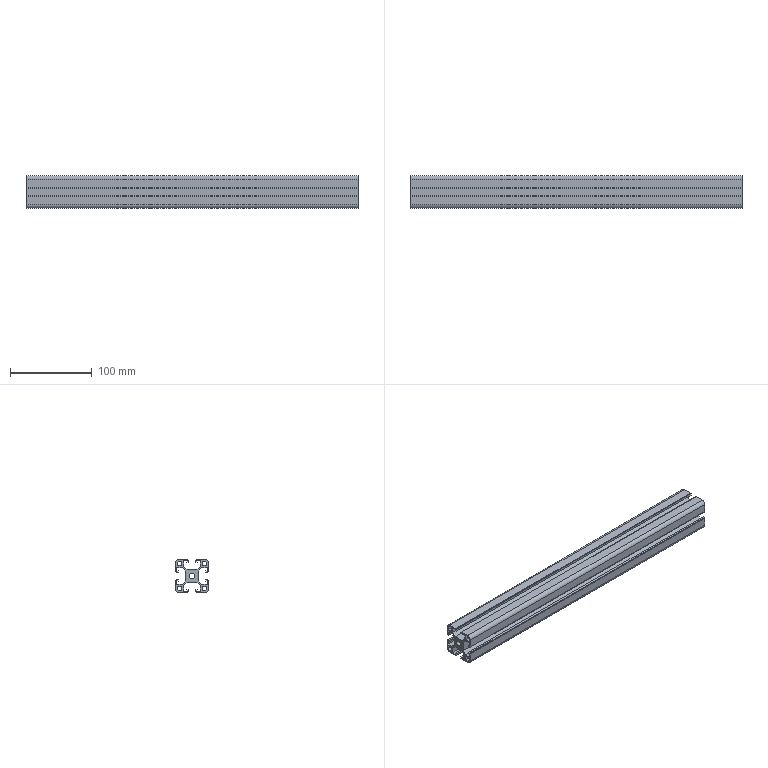Part | 1 solid | 104 faces | box 405 x 40 x 40 mm | volume 233501 mm3 | plane 94 | cylinder 10 | commonest cylinder face diameters 5 x4 9 x4 6.8 x2